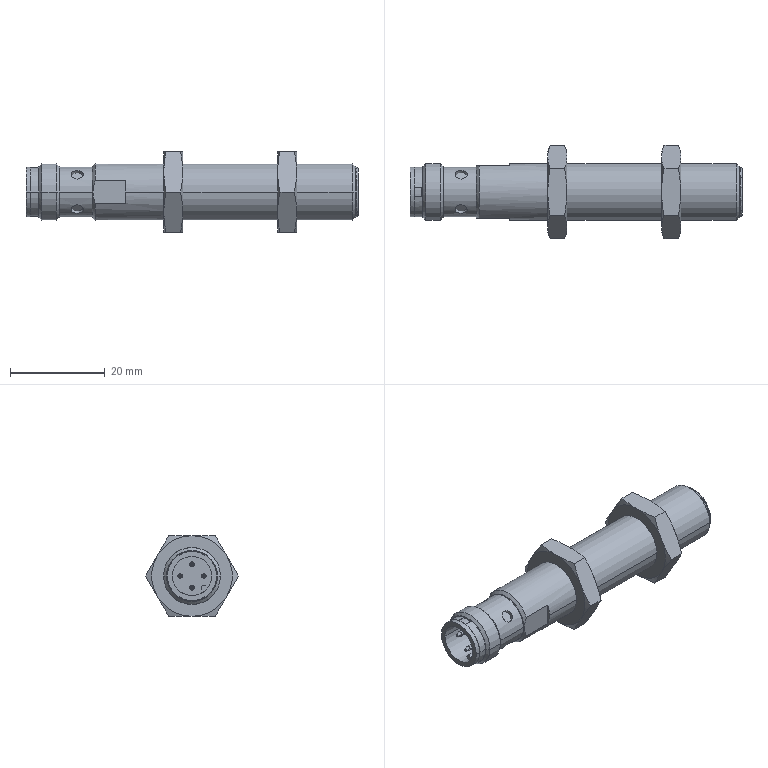Part | 1 solid | 127 faces | box 70 x 19.63 x 17 mm | volume 8211 mm3 | plane 48 | cone 42 | cylinder 35 | torus 2 | commonest cylinder face diameters 1 x8 2.5 x8 12 x8 10.5 x4 8.3 x2 10.3 x2